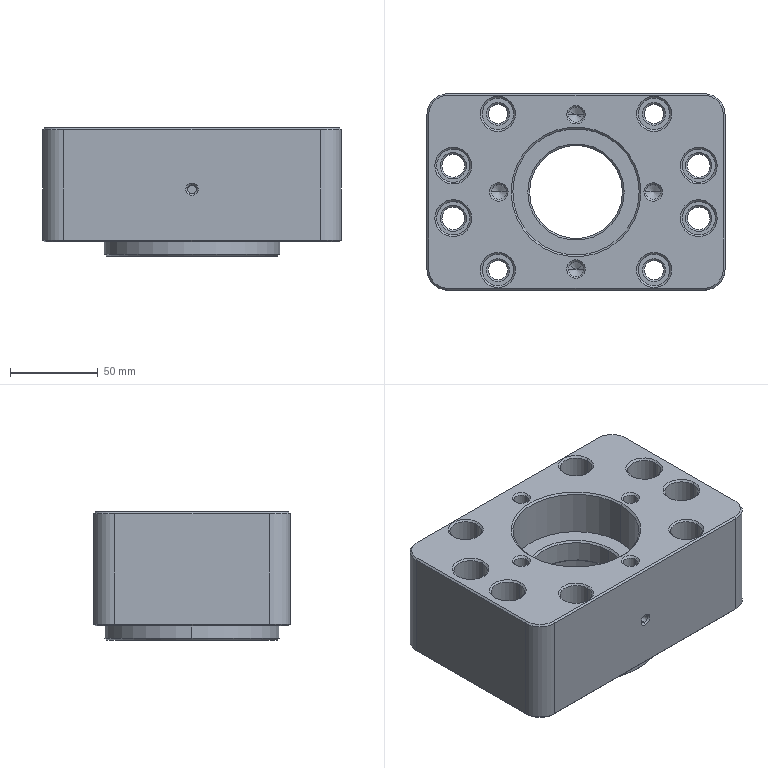NC program | NX | posted with a generic post | part box 170 x 112 x 73 mm
Lines 11425 to 12427 of 12427:
(FLOOR_WALL_1 , TOOL : D10JING)
N22830 T09 M6
N22832 G54
N22834 G17 G0 G90 X-74.428 Y61.442 S5000 M3
N22836 G43 Z30. H9
N22838 Z-6.5
N22840 G94 G1 Z-8. F1250.
N22842 X-73.885 Y60.5
N22844 G3 X-73.019 Y60. R1.
N22846 G1 X73.019
N22848 G2 X84.452 Y55.174 R16.
N22850 G1 X6.87
N22852 G2 X23.589 Y50.348 R55.6
N22854 G1 X87.687
N22856 G2 X88.927 Y45.522 R16.
N22858 G1 X31.924
N22860 G2 X37.884 Y40.696 R55.6
N22862 G1 X89.
N22864 Y35.87
N22866 X42.482
N22868 G2 X46.127 Y31.043 R55.6
N22870 G1 X89.
N22872 Y26.217
N22874 X49.031
N22876 G2 X51.32 Y21.391 R55.6
N22878 G1 X89.
N22880 Y16.565
N22882 X53.075
N22884 G2 X54.347 Y11.739 R55.6
N22886 G1 X89.
N22888 Y6.913
N22890 X55.169
N22892 G2 X55.561 Y2.087 R55.6
N22894 G1 X89.
N22896 Y-2.739
N22898 X55.532
N22900 G2 X55.083 Y-7.565 R55.6
N22902 G1 X89.
N22904 Y-12.391
N22906 X54.202
N22908 G2 X52.867 Y-17.217 R55.6
N22910 G1 X89.
N22912 Y-22.043
N22914 X51.044
N22916 G2 X48.676 Y-26.87 R55.6
N22918 G1 X89.
N22920 Y-31.696
N22922 X45.681
N22924 G2 X41.923 Y-36.522 R55.6
N22926 G1 X89.
N22928 Y-41.348
N22930 X37.171
N22932 G2 X30.973 Y-46.174 R55.6
N22934 G1 X88.852
N22936 G2 X87.388 Y-51. R16.
N22938 G1 X22.144
N22940 Z-6.5
N22942 G0 Z30.
N22944 X6.87 Y55.174
N22946 Z-6.5
N22948 G1 Z-8.
N22950 G3 X-6.87 Y55.174 R55.6
N22952 G1 X-84.452
N22954 G3 X-87.687 Y50.348 R16.
N22956 G1 X-23.589
N22958 G3 X-31.924 Y45.522 R55.6
N22960 G1 X-88.927
N22962 G3 X-89. Y44. R16.
N22964 G1 Y40.696
N22966 X-37.884
N22968 G3 X-42.482 Y35.87 R55.6
N22970 G1 X-89.
N22972 Y31.043
N22974 X-46.127
N22976 G3 X-49.031 Y26.217 R55.6
N22978 G1 X-89.
N22980 Y21.391
N22982 X-51.32
N22984 G3 X-53.075 Y16.565 R55.6
N22986 G1 X-89.
N22988 Y11.739
N22990 X-54.347
N22992 G3 X-55.169 Y6.913 R55.6
N22994 G1 X-89.
N22996 Y2.087
N22998 X-55.561
N23000 G3 X-55.532 Y-2.739 R55.6
N23002 G1 X-89.
N23004 Y-7.565
N23006 X-55.083
N23008 G3 X-54.202 Y-12.391 R55.6
N23010 G1 X-89.
N23012 Y-17.217
N23014 X-52.867
N23016 G3 X-51.044 Y-22.043 R55.6
N23018 G1 X-89.
N23020 Y-26.87
N23022 X-48.676
N23024 G3 X-45.681 Y-31.696 R55.6
N23026 G1 X-89.
N23028 Y-36.522
N23030 X-41.923
N23032 G3 X-37.171 Y-41.348 R55.6
N23034 G1 X-89.
N23036 Y-44.
N23038 G3 X-88.852 Y-46.174 R16.
N23040 G1 X-30.973
N23042 G3 X-22.144 Y-51. R55.6
N23044 G1 X-87.388
N23046 G3 X-83.777 Y-55.826 R16.
N23048 G1 X83.777
N23050 G3 X84.643 Y-55.326 R1.
N23052 G1 X85.544 Y-56.202
N23054 Z-6.5
N23056 G0 Z30.
N23058 X1.717 Y-57.074
N23060 Z-6.5
N23062 G1 Z-8.
N23064 X0.866 Y-55.6
N23066 G3 X0. Y-55.1 R1.
N23068 G2 X-55.1 Y0. R55.1
N23070 X0. Y-55.1 R-55.1
N23072 G3 X-0.866 Y-55.6 R1.
N23074 G1 X-1.717 Y-57.074
N23076 Z-6.5
N23078 G0 Z30.
N23080 X0.848 Y33.9
N23082 Z-30.5
N23084 G1 Z-32.
N23086 G3 X-0.019 Y34.4 R1.
N23088 G1 X0.017
N23090 G2 X17.718 Y29.486 R34.4
N23092 G1 X-17.719 Y29.485
N23094 G3 X-24.076 Y24.571 R34.4
N23096 G1 X24.074 Y24.572
N23098 G2 X28.23 Y19.658 R34.4
N23100 G1 X-28.231 Y19.656
N23102 G3 X-31.081 Y14.742 R34.4
N23104 G1 X31.08 Y14.744
N23106 G2 X32.966 Y9.829 R34.4
N23108 G1 X-32.966 Y9.828
N23110 G3 X-34.047 Y4.913 R34.4
N23112 G1 X34.047 Y4.915
N23114 G2 X34.4 Y0.001 R34.4
N23116 G1 X-34.4 Y-0.001
N23118 G3 X-34.047 Y-4.915 R34.4
N23120 G1 X34.047 Y-4.913
N23122 G2 X32.966 Y-9.828 R34.4
N23124 G1 X-32.966 Y-9.829
N23126 G3 X-31.08 Y-14.744 R34.4
N23128 G1 X31.081 Y-14.742
N23130 G2 X28.231 Y-19.656 R34.4
N23132 G1 X-28.23 Y-19.658
N23134 G3 X-24.074 Y-24.572 R34.4
N23136 G1 X24.076 Y-24.571
N23138 G2 X17.719 Y-29.485 R34.4
N23140 G1 X-17.718 Y-29.486
N23142 G3 X-0.017 Y-34.4 R34.4
N23144 G1 X0.019
N23146 G3 X0.885 Y-33.9 R1.
N23148 G1 X-0.847 Y-34.4
N23150 G3 X0.019 Y-34.9 R1.
N23152 X34.9 Y0.019 R34.9
N23154 X0.019 Y-34.9 R-34.9
N23156 X0.885 Y-34.4 R1.
N23158 G1 X1.48 Y-33.367
N23160 Z-30.5
N23162 G0 Z30.
(ZLEVEL_PROFILE_COPY , TOOL : D10JING)
N23164 X1.166 Y34.981
N23166 Z-8.
N23168 G1 X0.866 Y35.5 F1000.
N23170 G3 X0. Y36. R1.
N23172 X-36. Y0. R36. F1200.
N23174 X0. Y36. R-36.
N23176 X-0.866 Y35.5 R1.
N23178 G1 X-1.166 Y34.981
N23180 G0 X1.166 Z-16.
N23182 G1 X0.866 Y35.5 F1000.
N23184 G3 X0. Y36. R1.
N23186 X-18.702 Y30.761 R36. F1200.
N23188 G1 X-18.71 Y30.744
N23190 X-18.721 Y30.749
N23192 G3 X-21.373 Y28.969 R36.
N23194 G1 X-21.365 Y28.959
N23196 X-21.371 Y28.948
N23198 X-21.383 Y28.949
N23200 X-21.395 Y28.953
N23202 G3 X-22.536 Y28.074 R36.
N23204 G1 X-22.53 Y28.066
N23206 X-22.54 Y28.07
N23208 G3 X-28.07 Y22.54 R36.
N23210 G1 X-28.066 Y22.53
N23212 X-28.074 Y22.536
N23214 G3 X-28.953 Y21.395 R36.
N23216 G1 X-28.951 Y21.389
N23218 X-28.945 Y21.376
N23220 X-28.957 Y21.366
N23222 X-28.969 Y21.373
N23224 G3 X-30.749 Y18.721 R36.
N23226 G1 X-30.744 Y18.71
N23228 X-30.761 Y18.702
N23230 G3 X-30.761 Y-18.702 R36.
N23232 G1 X-30.744 Y-18.71
N23234 X-30.749 Y-18.721
N23236 G3 X-28.969 Y-21.373 R36.
N23238 G1 X-28.959 Y-21.365
N23240 X-28.948 Y-21.371
N23242 X-28.949 Y-21.383
N23244 X-28.953 Y-21.395
N23246 G3 X-28.074 Y-22.536 R36.
N23248 G1 X-28.066 Y-22.53
N23250 X-28.07 Y-22.54
N23252 G3 X-22.54 Y-28.07 R36.
N23254 G1 X-22.53 Y-28.066
N23256 X-22.536 Y-28.074
N23258 G3 X-21.395 Y-28.953 R36.
N23260 G1 X-21.389 Y-28.951
N23262 X-21.376 Y-28.945
N23264 X-21.366 Y-28.957
N23266 X-21.373 Y-28.969
N23268 G3 X-18.721 Y-30.749 R36.
N23270 G1 X-18.71 Y-30.744
N23272 X-18.702 Y-30.761
N23274 G3 X18.702 Y-30.761 R36.
N23276 G1 X18.71 Y-30.744
N23278 X18.721 Y-30.749
N23280 G3 X21.373 Y-28.969 R36.
N23282 G1 Y-28.963
N23284 X21.372 Y-28.949
N23286 X21.385 Y-28.942
N23288 X21.395 Y-28.953
N23290 G3 X22.536 Y-28.074 R36.
N23292 G1 X22.53 Y-28.066
N23294 X22.54 Y-28.07
N23296 G3 X28.07 Y-22.54 R36.
N23298 G1 X28.066 Y-22.53
N23300 X28.074 Y-22.536
N23302 G3 X28.953 Y-21.395 R36.
N23304 G1 X28.942 Y-21.388
N23306 X28.944 Y-21.375
N23308 X28.957 Y-21.373
N23310 X28.969
N23312 G3 X30.749 Y-18.721 R36.
N23314 G1 X30.744 Y-18.71
N23316 X30.761 Y-18.702
N23318 G3 X30.761 Y18.702 R36.
N23320 G1 X30.744 Y18.71
N23322 X30.749 Y18.721
N23324 G3 X28.969 Y21.373 R36.
N23326 G1 X28.959 Y21.365
N23328 X28.948 Y21.371
N23330 X28.949 Y21.383
N23332 X28.953 Y21.395
N23334 G3 X28.074 Y22.536 R36.
N23336 G1 X28.066 Y22.53
N23338 X28.07 Y22.54
N23340 G3 X22.54 Y28.07 R36.
N23342 G1 X22.53 Y28.066
N23344 X22.536 Y28.074
N23346 G3 X21.395 Y28.953 R36.
N23348 G1 X21.388 Y28.942
N23350 X21.375 Y28.944
N23352 X21.373 Y28.957
N23354 Y28.969
N23356 G3 X18.721 Y30.749 R36.
N23358 G1 X18.71 Y30.744
N23360 X18.702 Y30.761
N23362 G3 X0. Y36. R36.
N23364 X-0.866 Y35.5 R1.
N23366 G1 X-1.166 Y34.981
N23368 G0 Z30.
N23370 M5
(ZLEVEL_PROFILE_1_COPY , TOOL : D3R0.5)
N23372 T05 M6
N23374 G54
N23376 G17 G0 G90 X0.522 Y38.893 S7000 M3
N23378 G43 Z30. H5
N23380 Z-15.297
N23382 G94 G1 Z-16.297 F2500.
N23384 X0.26 Y39.346
N23386 G3 X0. Y39.496 R0.3
N23388 X-39.496 Y0. R39.496
N23390 X0. Y39.496 R-39.496
N23392 G1 Y39.461 Z-16.332
N23394 G2 X39.461 Y0. R39.461
N23396 X0. Y39.461 R-39.461
N23398 G1 Y39.426 Z-16.367
N23400 G3 X-39.426 Y0. R39.426
N23402 X0. Y39.426 R-39.426
N23404 G1 Y39.39 Z-16.403
N23406 G2 X39.39 Y0. R39.39
N23408 X0. Y39.39 R-39.39
N23410 G1 Y39.355 Z-16.438
N23412 G3 X-39.355 Y0. R39.355
N23414 X0. Y39.355 R-39.355
N23416 G1 Y39.32 Z-16.473
N23418 G2 X39.32 Y0. R39.32
N23420 X0. Y39.32 R-39.32
N23422 G1 Y39.284 Z-16.509
N23424 G3 X-39.284 Y0. R39.284
N23426 X0. Y39.284 R-39.284
N23428 G1 Y39.249 Z-16.544
N23430 G2 X39.249 Y0. R39.249
N23432 X0. Y39.249 R-39.249
N23434 G1 Y39.214 Z-16.579
N23436 G3 X-39.214 Y0. R39.214
N23438 X0. Y39.214 R-39.214
N23440 G1 Y39.178 Z-16.615
N23442 G2 X39.178 Y0. R39.178
N23444 X0. Y39.178 R-39.178
N23446 G1 Y39.143 Z-16.65
N23448 G3 X-39.143 Y0. R39.143
N23450 X0. Y39.143 R-39.143
N23452 G1 Y39.107 Z-16.685
N23454 G2 X39.107 Y0. R39.107
N23456 X0. Y39.107 R-39.107
N23458 G1 Y39.072 Z-16.721
N23460 G3 X-39.072 Y0. R39.072
N23462 X0. Y39.072 R-39.072
N23464 G1 Y39.037 Z-16.756
N23466 G2 X39.037 Y0. R39.037
N23468 X0. Y39.037 R-39.037
N23470 G1 Y39.001 Z-16.791
N23472 G3 X-39.001 Y0. R39.001
N23474 X0. Y39.001 R-39.001
N23476 G1 Y38.966 Z-16.827
N23478 G2 X38.966 Y0. R38.966
N23480 X0. Y38.966 R-38.966
N23482 G1 Y38.931 Z-16.862
N23484 G3 X-38.931 Y0. R38.931
N23486 X0. Y38.931 R-38.931
N23488 G1 Y38.895 Z-16.898
N23490 G2 X38.895 Y0. R38.895
N23492 X0. Y38.895 R-38.895
N23494 G1 Y38.86 Z-16.933
N23496 G3 X-38.86 Y0. R38.86
N23498 X0. Y38.86 R-38.86
N23500 G1 Y38.825 Z-16.968
N23502 G2 X38.825 Y0. R38.825
N23504 X0. Y38.825 R-38.825
N23506 G1 Y38.789 Z-17.004
N23508 G3 X-38.789 Y0. R38.789
N23510 X0. Y38.789 R-38.789
N23512 G1 Y38.754 Z-17.039
N23514 G2 X38.754 Y0. R38.754
N23516 X0. Y38.754 R-38.754
N23518 G1 Y38.719 Z-17.074
N23520 G3 X-38.719 Y0. R38.719
N23522 X0. Y38.719 R-38.719
N23524 G1 Y38.683 Z-17.11
N23526 G2 X38.683 Y0. R38.683
N23528 X0. Y38.683 R-38.683
N23530 G1 Y38.648 Z-17.145
N23532 G3 X-2.08 Y38.592 R38.648
N23534 G1 X-2.324 Y38.578
N23536 G3 X-2.569 Y38.562 R38.648
N23538 G1 X-2.97 Y38.534
N23540 G3 X-3.303 Y38.506 R38.648
N23542 G1 X-3.792 Y38.461
N23544 G3 X-8.685 Y37.659 R38.648
N23546 G1 X-8.93 Y37.602
N23548 G3 X-10.398 Y37.223 R38.648
N23550 G1 X-10.642 Y37.154
N23552 G3 X-12.111 Y36.701 R38.648
N23554 G1 X-12.355 Y36.62
N23556 G3 X-13.579 Y36.184 R38.648
N23558 G1 X-13.834 Y36.087
N23560 G3 X-15.052 Y35.596 R38.648
N23562 G1 X-15.535 Y35.388
N23564 G3 X-16.514 Y34.942 R38.648
N23566 G1 X-17.003 Y34.703
N23568 Y34.705
N23570 X-16.679 Y34.864
N23572 G3 X-18.472 Y33.948 R38.648
N23574 G1 X-18.133 Y34.128
N23576 X-18.128
N23578 X-18.587 Y33.885
N23580 G3 X-19.205 Y33.538 R38.648
N23582 G1 X-19.452 Y33.396
N23584 G3 X-20.918 Y32.498 R38.648
N23586 G1 X-21.463 Y32.136
N23588 X-21.415 Y32.173
N23590 G3 X-22.386 Y31.504 R38.648
N23592 G1 X-22.906 Y31.124
N23594 X-22.875 Y31.15
N23596 X-22.478 Y31.438
N23598 G3 X-24.099 Y30.214 R38.648
N23600 G1 X-23.787 Y30.459
N23602 X-23.752 Y30.483
N23604 X-24.343 Y30.018
N23606 G3 X-24.992 Y29.48 R38.648
N23608 G1 X-25.583 Y28.964
N23610 X-25.566 Y28.984
N23612 G3 X-26.478 Y28.152 R38.648
N23614 G1 X-26.3 Y28.317
N23616 X-26.287 Y28.327
N23618 X-26.881 Y27.769
N23620 G3 X-27.62 Y27.034 R38.648
N23622 G1 X-27.523 Y27.13
N23624 Y27.126
N23626 X-28.089 Y26.545
N23628 G3 X-28.766 Y25.81 R38.648
N23630 G1 X-28.746 Y25.83
N23632 Y25.825
N23634 X-29.236 Y25.277
N23636 G3 X-29.726 Y24.699 R38.648
N23638 G1 X-30.293 Y23.994
N23640 X-30.214 Y24.099
N23642 G3 X-30.786 Y23.364 R38.648
N23644 G1 X-31.335 Y22.617
N23646 X-31.276 Y22.704
N23648 G3 X-31.847 Y21.896 R38.648
N23650 G1 X-31.796 Y21.964
N23652 X-32.326 Y21.177
N23654 X-32.277 Y21.257
N23656 G3 X-32.739 Y20.538 R38.648
N23658 G1 X-32.679 Y20.628
N23660 X-33.212 Y19.757
N23662 X-33.15 Y19.868
N23664 G3 X-33.64 Y19.026 R38.648
N23666 G1 X-33.572 Y19.139
N23668 X-34.08 Y18.227
N23670 G3 X-34.408 Y17.6 R38.648
N23672 G1 X-34.373 Y17.665
N23674 Y17.66
N23676 X-34.838 Y16.724
N23678 X-34.825 Y16.759
N23680 G3 X-35.16 Y16.045 R38.648
N23682 G1 X-35.107 Y16.157
N23684 Y16.152
N23686 X-35.489 Y15.291
N23688 X-35.559 Y15.14
N23690 G3 X-35.82 Y14.511 R38.648
N23692 G1 X-35.777 Y14.609
N23694 X-36.186 Y13.564
N23696 X-36.164 Y13.63
N23698 G3 X-36.388 Y13.023 R38.648
N23700 G1 X-36.365 Y13.079
N23702 X-36.781 Y11.866
N23704 G3 X-36.936 Y11.376 R38.648
N23706 G1 X-36.915 Y11.43
N23708 X-37.223 Y10.398
N23710 G3 X-37.356 Y9.908 R38.648
N23712 G1 X-37.414 Y9.664
N23714 X-37.661 Y8.661
N23716 X-37.659 Y8.685
N23718 G3 X-37.769 Y8.196 R38.648
N23720 G1 X-37.798 Y8.032
N23722 X-38.014 Y6.973
N23724 G3 X-38.1 Y6.483 R38.648
N23726 G1 X-38.083 Y6.566
N23728 X-38.288 Y5.244
N23730 Y5.265
N23732 G3 X-38.333 Y4.925 R38.648
N23734 G1 X-38.347 Y4.771
N23736 X-38.481 Y3.558
N23738 X-38.48 Y3.603
N23740 G3 X-38.514 Y3.21 R38.648
N23742 G1 X-38.507 Y3.275
N23744 X-38.586 Y2.08
N23746 X-38.604 Y1.835
N23748 G3 X-38.617 Y1.535 R38.648
N23750 G1 X-38.613 Y1.577
N23752 X-38.645 Y0.129
N23754 X-38.647 Y0.172
N23756 G3 X-38.647 Y-0.172 R38.648
N23758 G1 X-38.645 Y-0.129
N23760 X-38.613 Y-1.577
N23762 X-38.617 Y-1.535
N23764 G3 X-38.604 Y-1.835 R38.648
N23766 G1 X-38.586 Y-2.08
N23768 X-38.507 Y-3.275
N23770 X-38.514 Y-3.21
N23772 G3 X-38.48 Y-3.603 R38.648
N23774 G1 X-38.481 Y-3.558
N23776 X-38.347 Y-4.771
N23778 X-38.333 Y-4.926
N23780 G3 X-38.288 Y-5.265 R38.648
N23782 G1 Y-5.244
N23784 X-38.083 Y-6.566
N23786 X-38.1 Y-6.483
N23788 G3 X-38.014 Y-6.973 R38.648
N23790 G1 X-37.798 Y-8.032
N23792 X-37.769 Y-8.196
N23794 G3 X-37.659 Y-8.685 R38.648
N23796 G1 X-37.661 Y-8.66
N23798 X-37.414 Y-9.664
N23800 X-37.356 Y-9.908
N23802 G3 X-37.223 Y-10.398 R38.648
N23804 G1 X-36.915 Y-11.43
N23806 X-36.936 Y-11.376
N23808 G3 X-36.781 Y-11.866 R38.648
N23810 G1 X-36.365 Y-13.079
N23812 X-36.388 Y-13.023
N23814 G3 X-36.164 Y-13.63 R38.648
N23816 G1 X-36.186 Y-13.564
N23818 X-35.777 Y-14.609
N23820 X-35.821 Y-14.509
N23822 G3 X-35.545 Y-15.172 R38.648
N23824 G1 X-35.489 Y-15.291
N23826 X-35.104 Y-16.159
N23828 X-35.107 Y-16.156
N23830 X-35.16 Y-16.046
N23832 G3 X-34.825 Y-16.759 R38.648
N23834 G1 X-34.839 Y-16.723
N23836 X-34.373 Y-17.66
N23838 Y-17.664
N23840 X-34.407 Y-17.601
N23842 G3 X-34.08 Y-18.227 R38.648
N23844 G1 X-33.575 Y-19.134
N23846 X-33.64 Y-19.026
N23848 G3 X-33.15 Y-19.868 R38.648
N23850 G1 X-33.212 Y-19.757
N23852 X-32.662 Y-20.66
N23854 G3 X-32.277 Y-21.257 R38.648
N23856 G1 X-32.326 Y-21.177
N23858 X-31.927 Y-21.769
N23860 X-31.847 Y-21.896
N23862 G3 X-31.274 Y-22.707 R38.648
N23864 G1 X-31.336 Y-22.615
N23866 X-30.786 Y-23.364
N23868 G3 X-30.214 Y-24.099 R38.648
N23870 G1 X-30.293 Y-23.994
N23872 X-29.726 Y-24.699
N23874 G3 X-29.236 Y-25.277 R38.648
N23876 G1 X-28.746 Y-25.825
N23878 Y-25.831
N23880 X-28.766 Y-25.81
N23882 G3 X-28.089 Y-26.545 R38.648
N23884 G1 X-27.523 Y-27.126
N23886 Y-27.13
N23888 X-27.62 Y-27.034
N23890 G3 X-26.881 Y-27.769 R38.648
N23892 G1 X-26.282 Y-28.331
N23894 X-26.3 Y-28.317
N23896 X-26.478 Y-28.152
N23898 G3 X-25.566 Y-28.984 R38.648
N23900 G1 X-25.586 Y-28.961
N23902 X-25.045 Y-29.43
N23904 X-25.077 Y-29.406
N23906 X-25.321 Y-29.197
N23908 G3 X-22.478 Y-31.438 R38.648
N23910 G1 X-22.875 Y-31.15
N23912 X-22.88 Y-31.143
N23914 X-22.386 Y-31.504
N23916 G3 X-21.415 Y-32.173 R38.648
N23918 G1 X-21.474 Y-32.129
N23920 X-21.038 Y-32.416
N23922 X-21.042
N23924 X-21.408 Y-32.177
N23926 G3 X-18.587 Y-33.885 R38.648
N23928 G1 X-18.128 Y-34.128
N23930 X-18.133
N23932 X-18.472 Y-33.948
N23934 G3 X-15.535 Y-35.388 R38.648
N23936 G1 X-15.052 Y-35.596
N23938 G3 X-13.834 Y-36.087 R38.648
N23940 G1 X-13.575 Y-36.182
N23942 X-13.578 Y-36.183
N23944 X-13.823 Y-36.091
N23946 G3 X-10.642 Y-37.154 R38.648
N23948 G1 X-10.398 Y-37.223
N23950 G3 X8.685 Y-37.659 R38.648
N23952 G1 X8.93 Y-37.602
N23954 G3 X10.398 Y-37.223 R38.648
N23956 G1 X10.642 Y-37.154
N23958 G3 X13.823 Y-36.091 R38.648
N23960 G1 X13.578 Y-36.183
N23962 X13.575 Y-36.182
N23964 X13.834 Y-36.087
N23966 G3 X15.052 Y-35.596 R38.648
N23968 G1 X15.535 Y-35.388
N23970 G3 X18.136 Y-34.128 R38.648
N23972 G1 X18.586 Y-33.885
N23974 G3 X21.408 Y-32.177 R38.648
N23976 G1 X21.042 Y-32.416
N23978 X21.038
N23980 X21.464 Y-32.135
N23982 X21.415 Y-32.173
N23984 G3 X22.386 Y-31.504 R38.648
N23986 G1 X22.88 Y-31.143
N23988 X22.875 Y-31.15
N23990 X22.478 Y-31.439
N23992 G3 X25.321 Y-29.197 R38.648
N23994 G1 X25.077 Y-29.406
N23996 X25.048 Y-29.427
N23998 X25.585 Y-28.962
N24000 X25.566 Y-28.984
N24002 G3 X26.479 Y-28.152 R38.648
N24004 G1 X26.3 Y-28.317
N24006 X26.283 Y-28.331
N24008 X26.881 Y-27.769
N24010 G3 X27.62 Y-27.034 R38.648
N24012 G1 X27.523 Y-27.13
N24014 X27.502 Y-27.148
N24016 X28.045 Y-26.587
N24018 X27.912 Y-26.731
N24020 G3 X28.766 Y-25.81 R38.648
N24022 G1 X28.658 Y-25.924
N24024 X29.236 Y-25.277
N24026 G3 X29.726 Y-24.699 R38.648
N24028 G1 X30.28 Y-24.01
N24030 X30.214 Y-24.099
N24032 G3 X30.786 Y-23.364 R38.648
N24034 G1 X31.33 Y-22.624
N24036 X31.328 Y-22.63
N24038 X31.272 Y-22.709
N24040 G3 X31.847 Y-21.896 R38.648
N24042 G1 X31.927 Y-21.769
N24044 X32.325 Y-21.178
N24046 X32.274 Y-21.262
N24048 G3 X32.653 Y-20.674 R38.648
N24050 G1 X33.211 Y-19.758
N24052 X33.15 Y-19.868
N24054 G3 X33.64 Y-19.026 R38.648
N24056 G1 X33.589 Y-19.108
N24058 X34.08 Y-18.227
N24060 G3 X34.405 Y-17.605 R38.648
N24062 G1 X34.373 Y-17.664
N24064 X34.369 Y-17.667
N24066 X34.838 Y-16.725
N24068 X34.825 Y-16.759
N24070 G3 X35.108 Y-16.157 R38.648
N24072 G1 X35.164 Y-16.024
N24074 X35.489 Y-15.291
N24076 X35.545 Y-15.172
N24078 G3 X35.821 Y-14.508 R38.648
N24080 G1 X35.778 Y-14.605
N24082 X36.185 Y-13.567
N24084 X36.164 Y-13.631
N24086 G3 X36.391 Y-13.015 R38.648
N24088 G1 X36.368 Y-13.069
N24090 X36.767 Y-11.903
N24092 X36.743 Y-11.984
N24094 G3 X36.936 Y-11.376 R38.648
N24096 G1 X36.911 Y-11.445
N24098 X37.24 Y-10.322
N24100 X37.223 Y-10.398
N24102 G3 X37.356 Y-9.908 R38.648
N24104 G1 X37.414 Y-9.664
N24106 X37.668 Y-8.632
N24108 X37.659 Y-8.685
N24110 G3 X37.788 Y-8.107 R38.648
N24112 G1 X37.767 Y-8.196
N24114 X37.763 Y-8.208
N24116 X37.962 Y-7.217
N24118 X38.014 Y-6.973
N24120 G3 X38.1 Y-6.483 R38.648
N24122 G1 X38.084 Y-6.56
N24124 X38.288 Y-5.244
N24126 Y-5.265
N24128 G3 X38.335 Y-4.909 R38.648
N24130 G1 X38.485 Y-3.548
N24132 G3 X38.515 Y-3.197 R38.648
N24134 G1 X38.508 Y-3.261
N24136 X38.601 Y-1.845
N24138 X38.602 Y-1.889
N24140 G3 X38.618 Y-1.528 R38.648
N24142 G1 X38.613 Y-1.569
N24144 X38.645 Y-0.129
N24146 X38.647 Y-0.17
N24148 G3 X38.647 Y0.17 R38.648
N24150 G1 X38.645 Y0.129
N24152 X38.613 Y1.569
N24154 X38.618 Y1.528
N24156 G3 X38.602 Y1.889 R38.648
N24158 G1 X38.601 Y1.845
N24160 X38.508 Y3.261
N24162 X38.515 Y3.197
N24164 G3 X38.485 Y3.548 R38.648
N24166 G1 X38.335 Y4.909
N24168 G3 X38.288 Y5.265 R38.648
N24170 G1 Y5.244
N24172 X38.084 Y6.56
N24174 X38.1 Y6.483
N24176 G3 X38.014 Y6.973 R38.648
N24178 G1 X37.962 Y7.217
N24180 X37.763 Y8.208
N24182 X37.767 Y8.196
N24184 X37.788 Y8.106
N24186 G3 X37.659 Y8.685 R38.648
N24188 G1 X37.668 Y8.632
N24190 X37.414 Y9.664
N24192 X37.356 Y9.908
N24194 G3 X37.223 Y10.398 R38.648
N24196 G1 X37.24 Y10.322
N24198 X36.911 Y11.445
N24200 X36.936 Y11.376
N24202 G3 X36.743 Y11.984 R38.648
N24204 G1 X36.767 Y11.903
N24206 X36.368 Y13.069
N24208 X36.391 Y13.015
N24210 G3 X36.164 Y13.631 R38.648
N24212 G1 X36.185 Y13.567
N24214 X35.778 Y14.604
N24216 X35.82 Y14.51
N24218 G3 X35.555 Y15.149 R38.648
N24220 G1 X35.489 Y15.291
N24222 X35.164 Y16.024
N24224 X35.108 Y16.157
N24226 G3 X34.825 Y16.759 R38.648
N24228 G1 X34.837 Y16.726
N24230 X34.37 Y17.667
N24232 X34.373 Y17.665
N24234 X34.406 Y17.604
N24236 G3 X34.08 Y18.227 R38.648
N24238 G1 X33.586 Y19.114
N24240 X33.64 Y19.026
N24242 G3 X33.15 Y19.868 R38.648
N24244 G1 X33.211 Y19.759
N24246 X32.68 Y20.627
N24248 X32.744 Y20.53
N24250 G3 X32.274 Y21.262 R38.648
N24252 G1 X32.325 Y21.178
N24254 X31.786 Y21.978
N24256 X31.847 Y21.896
N24258 G3 X31.275 Y22.706 R38.648
N24260 G1 X31.328 Y22.63
N24262 X31.329 Y22.624
N24264 X30.786 Y23.364
N24266 G3 X30.214 Y24.099 R38.648
N24268 G1 X30.28 Y24.01
N24270 X29.726 Y24.699
N24272 G3 X29.236 Y25.277 R38.648
N24274 G1 X28.663 Y25.92
N24276 X28.766 Y25.81
N24278 G3 X28.089 Y26.545 R38.648
N24280 G1 X27.503 Y27.147
N24282 X27.523 Y27.13
N24284 X27.62 Y27.034
N24286 G3 X26.881 Y27.769 R38.648
N24288 G1 X26.287 Y28.326
N24290 X26.3 Y28.317
N24292 X26.478 Y28.152
N24294 G3 X25.566 Y28.984 R38.648
N24296 G1 X25.583 Y28.964
N24298 X24.992 Y29.48
N24300 G3 X24.343 Y30.018 R38.648
N24302 G1 X23.752 Y30.483
N24304 X23.787 Y30.459
N24306 X24.099 Y30.214
N24308 G3 X22.478 Y31.439 R38.648
N24310 G1 X22.875 Y31.15
N24312 X22.906 Y31.124
N24314 X22.386 Y31.504
N24316 G3 X21.415 Y32.173 R38.648
N24318 G1 X21.454 Y32.141
N24320 X20.918 Y32.498
N24322 G3 X19.452 Y33.396 R38.648
N24324 G1 X19.205 Y33.538
N24326 G3 X18.586 Y33.885 R38.648
N24328 G1 X18.136 Y34.128
N24330 G3 X15.535 Y35.388 R38.648
N24332 G1 X15.052 Y35.596
N24334 G3 X13.834 Y36.087 R38.648
N24336 G1 X13.579 Y36.184
N24338 G3 X12.355 Y36.62 R38.648
N24340 G1 X12.111 Y36.701
N24342 G3 X10.642 Y37.154 R38.648
N24344 G1 X10.398 Y37.223
N24346 G3 X8.93 Y37.602 R38.648
N24348 G1 X8.685 Y37.659
N24350 G3 X3.792 Y38.461 R38.648
N24352 G1 X3.303 Y38.506
N24354 G3 X2.97 Y38.534 R38.648
N24356 G1 X2.569 Y38.562
N24358 G3 X2.324 Y38.578 R38.648
N24360 G1 X2.08 Y38.592
N24362 G3 X0. Y38.648 R38.648
N24364 G1 Y38.61 Z-17.18
N24366 G2 X38.61 Y0. R38.61
N24368 X0. Y38.61 R-38.61
N24370 G1 Y38.576 Z-17.216
N24372 G3 X-38.575 Y0. R38.575
N24374 X0. Y38.576 R-38.575
N24376 G1 Y38.539 Z-17.251
N24378 G2 X38.538 Y-0.001 R38.539
N24380 X0. Y38.539 R-38.539
N24382 G1 Y38.523 Z-17.269
N24384 Y38.504 Z-17.286
N24386 G3 X-38.505 Y0.001 R38.504
N24388 X0. Y38.504 R-38.504
N24390 G1 Y38.488 Z-17.304
N24392 Y38.469 Z-17.322
N24394 G2 X38.469 Y0. R38.469
N24396 X0. Y38.469 R-38.469
N24398 G1 Y38.453 Z-17.339
N24400 Y38.433 Z-17.357
N24402 G3 X-38.434 Y-0.001 R38.434
N24404 X0. Y38.433 R-38.434
N24406 G1 Y38.417 Z-17.375
N24408 Y38.398 Z-17.393
N24410 G2 X38.398 Y0. R38.398
N24412 X0. Y38.398 R-38.398
N24414 G1 Y38.382 Z-17.41
N24416 Y38.362 Z-17.428
N24418 G3 X-38.362 Y0. R38.362
N24420 X0. Y38.362 R-38.362
N24422 G1 Y38.346 Z-17.446
N24424 Y38.327 Z-17.463
N24426 G2 X38.327 Y0. R38.327
N24428 X0. Y38.327 R-38.327
N24430 G1 Y38.31 Z-17.482
N24432 Y38.29 Z-17.5
N24434 G3 X-38.29 Y0. R38.29
N24436 X0. Y38.29 R-38.29
N24438 X-0.26 Y38.14 R0.3
N24440 G1 X-0.522 Y37.686
N24442 Z-16.5
N24444 G0 Z30.
N24446 M5
(DRILLING_COPY_1_COPY , TOOL : D6A45)
N24448 T07 M6
N24450 G54
N24452 G17 G0 G90 X42.426 Y-15. S5000 M3
N24454 G43 Z30. H7
N24456 G94 G81 G98 Z-2.65 F250. R3.
N24458 Y15.
N24460 X-42.426
N24462 Y-15.
N24464 G80
N24466 G0 X-42.426 Y-15. Z30.
(PLANAR_MILL_1_COPY_COPY_1 , TOOL : D6A45)
N24468 X-51.3 Y-0.866 S7500
N24470 Z1.2
N24472 G1 Z-1.8 F1250.
N24474 G3 X-50.8 Y0. R1.
N24476 G2 X0. Y50.8 R50.8
N24478 X-50.8 Y0. R-50.8
N24480 G3 X-51.3 Y0.866 R1.
N24482 G1 Z1.2
N24484 G0 Z30.
N24486 X-39.7
N24488 Z1.2
N24490 G1 Z-1.8
N24492 G3 X-40.2 Y0. R1.
N24494 X0. Y-40.2 R40.2
N24496 X-40.2 Y0. R-40.2
N24498 X-39.7 Y-0.866 R1.
N24500 G1 Z1.2
N24502 G0 Z30.
(PLANAR_MILL_1_COPY_COPY_1_COPY , TOOL : D6A45)
N24504 X43.634 Y-48.7
N24506 Z-6.8
N24508 G1 Z-9.8
N24510 G3 X44.5 Y-49.2 R1.
N24512 X49.2 Y-44.5 R4.7
N24514 X44.5 Y-49.2 R-4.7
N24516 X45.366 Y-48.7 R1.
N24518 G1 Z-6.8
N24520 G0 Z30.
N24522 X75.2 Y-15.866
N24524 Z-6.8
N24526 G1 Z-9.8
N24528 G3 X75.7 Y-15. R1.
N24530 X70. Y-9.3 R5.7
N24532 X75.7 Y-15. R-5.7
N24534 X75.2 Y-14.134 R1.
N24536 G1 Z-6.8
N24538 G0 Z30.
N24540 Y14.134
N24542 Z-6.8
N24544 G1 Z-9.8
N24546 G3 X75.7 Y15. R1.
N24548 X70. Y20.7 R5.7
N24550 X75.7 Y15. R-5.7
N24552 X75.2 Y15.866 R1.
N24554 G1 Z-6.8
N24556 G0 Z30.
N24558 X45.366 Y48.7
N24560 Z-6.8
N24562 G1 Z-9.8
N24564 G3 X44.5 Y49.2 R1.
N24566 X39.8 Y44.5 R4.7
N24568 X44.5 Y49.2 R-4.7
N24570 X43.634 Y48.7 R1.
N24572 G1 Z-6.8
N24574 G0 Z30.
N24576 X-0.866 Y57.3
N24578 Z-6.8
N24580 G1 Z-9.8
N24582 G3 X0. Y56.8 R1.
N24584 G1 X73.
N24586 G2 X85.8 Y44. R12.8
N24588 G1 Y-44.
N24590 G2 X73. Y-56.8 R12.8
N24592 G1 X-73.
N24594 G2 X-85.8 Y-44. R12.8
N24596 G1 Y44.
N24598 G2 X-73. Y56.8 R12.8
N24600 G1 X0.
N24602 G3 X0.866 Y57.3 R1.
N24604 G1 Z-6.8
N24606 G0 Z30.
N24608 X-43.634 Y48.7
N24610 Z-6.8
N24612 G1 Z-9.8
N24614 G3 X-44.5 Y49.2 R1.
N24616 X-49.2 Y44.5 R4.7
N24618 X-44.5 Y49.2 R-4.7
N24620 X-45.366 Y48.7 R1.
N24622 G1 Z-6.8
N24624 G0 Z30.
N24626 X-75.2 Y15.866
N24628 Z-6.8
N24630 G1 Z-9.8
N24632 G3 X-75.7 Y15. R1.
N24634 X-70. Y9.3 R5.7
N24636 X-75.7 Y15. R-5.7
N24638 X-75.2 Y14.134 R1.
N24640 G1 Z-6.8
N24642 G0 Z30.
N24644 Y-14.134
N24646 Z-6.8
N24648 G1 Z-9.8
N24650 G3 X-75.7 Y-15. R1.
N24652 X-70. Y-20.7 R5.7
N24654 X-75.7 Y-15. R-5.7
N24656 X-75.2 Y-15.866 R1.
N24658 G1 Z-6.8
N24660 G0 Z30.
N24662 X-45.366 Y-48.7
N24664 Z-6.8
N24666 G1 Z-9.8
N24668 G3 X-44.5 Y-49.2 R1.
N24670 X-39.8 Y-44.5 R4.7
N24672 X-44.5 Y-49.2 R-4.7
N24674 X-43.634 Y-48.7 R1.
N24676 G1 Z-6.8
N24678 G0 Z30.
N24680 M5
(刀补 , TOOL : D10JING)
N24682 T09 M6
N24684 G54
N24686 G17 G0 G90 X-1.496 Y-33.324 S5000 M3
N24688 G43 Z30. H9
N24690 Z-30.5
N24692 G94 G1 Z-32. F1250.
N24694 G41 X-1.462 Y-33.418 D9
N24696 X-0.866 Y-34.45
N24698 G3 X0. Y-34.95 R1.
N24700 X34.95 Y0. R34.95
N24702 X0. Y-34.95 R-34.95
N24704 X0.866 Y-34.45 R1.
N24706 G1 X1.462 Y-33.418
N24708 G40
N24710 X1.496 Y-33.324
N24712 Z-30.5
N24714 G0 Z30.
N24716 M5
(PLANAR_MILL_1_COPY_COPY_1_COPY_COPY , TOOL : D6A45)
N24718 T07 M6
N24720 G54
N24722 G17 G0 G90 X-25.2 Y0.866 S7500 M3
N24724 G43 Z30. H7
N24726 Z-30.8
N24728 G94 G1 Z-33.8 F1250.
N24730 G3 X-25.7 Y0. R1.
N24732 X0. Y-25.7 R25.7
N24734 X-25.7 Y0. R-25.7
N24736 X-25.2 Y-0.866 R1.
N24738 G1 Z-30.8
N24740 G0 Z30.
N24742 M5
(刀补_COPY , TOOL : D10JING)
N24744 T09 M6
N24746 G54
N24748 G17 G0 G90 X1.467 Y-56.626 S5000 M3
N24750 G43 Z30. H9
N24752 Z-6.5
N24754 G94 G1 Z-8. F1250.
N24756 G41 X1.433 Y-56.532 D9
N24758 X0.866 Y-55.55
N24760 G3 X0. Y-55.05 R1.
N24762 G2 X-55.05 Y0. R55.05
N24764 X0. Y-55.05 R-55.05
N24766 G3 X-0.866 Y-55.55 R1.
N24768 G1 X-1.433 Y-56.532
N24770 G40
N24772 X-1.467 Y-56.626
N24774 Z-6.5
N24776 G0 Z30.
N24778 M5
N24780 M2